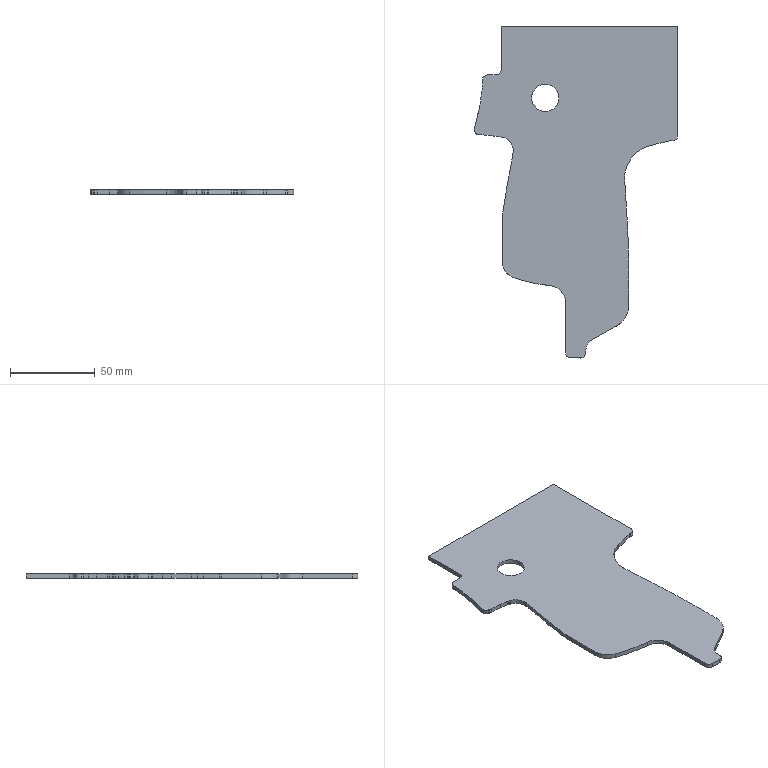Part | STEP file | lll_id1246_x_t | 1 solid | 77 faces | box 120.313 x 196.141 x 2.5 mm | volume 36784 mm3 | cylinder 67 | plane 10 | commonest cylinder face diameters 6 x7 20 x3 380.779 x2 5.007 x1 5.202 x1 6.807 x1